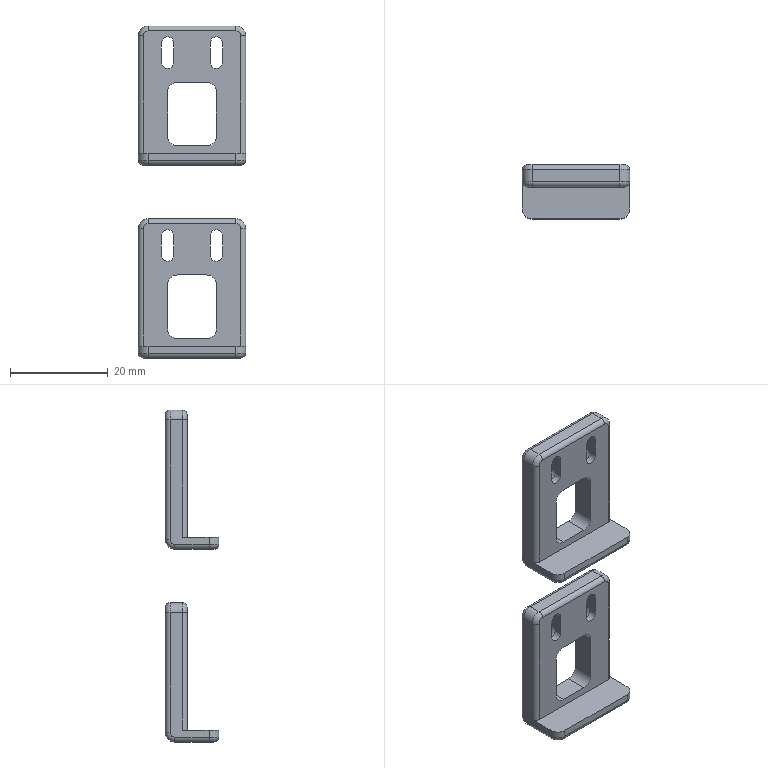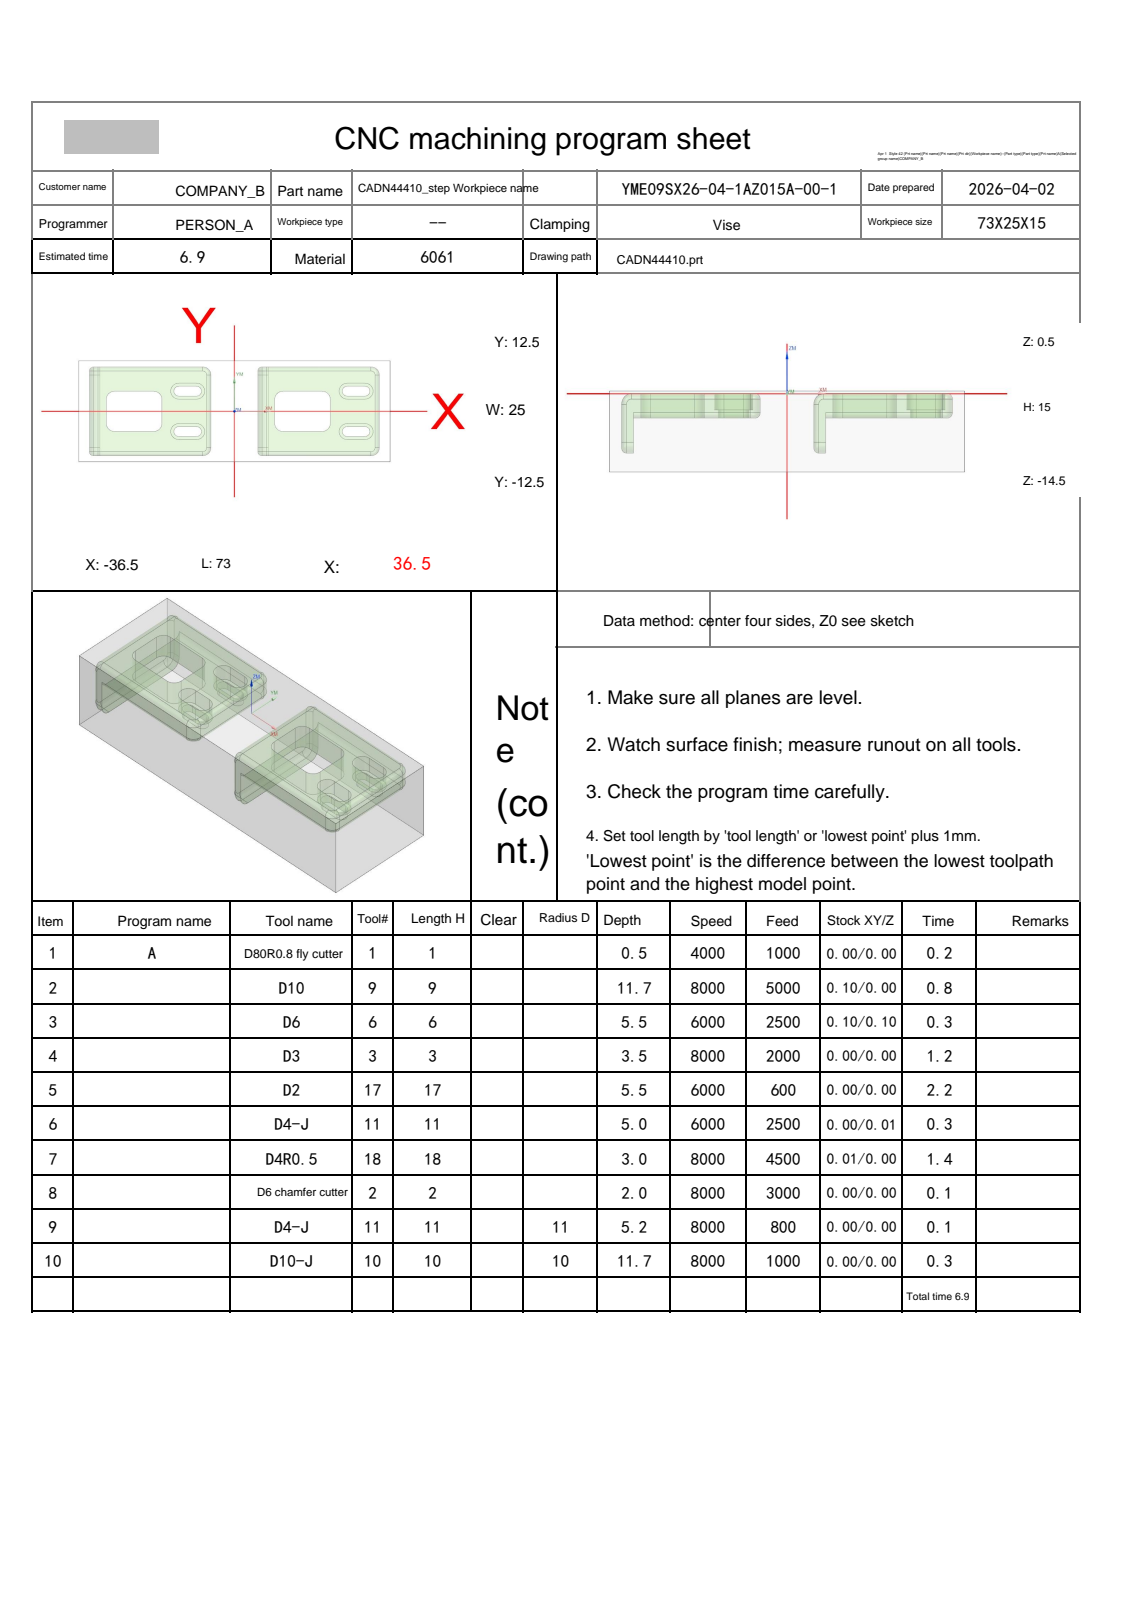NC program | NX | posted by the shop | part box 22 x 11 x 68 mm
Lines 3075 to 4128 of 7842:
N6 T11 M06
(D4-J  D=4. R=0. H=11 ce=0.00 di=0.01)
G00 G90 G54 X-26.358 Y2.4 M03 S6000
G43 H11 Z20.
M08
Z.319
G01 X-26.359 Y2.407 Z.233 F2000.
X-26.362 Y2.426 Z.155
X-26.367 Y2.455 Z.085
X-26.375 Y2.494 Z.023
X-26.386 Y2.539 Z-.033
X-26.4 Y2.59 Z-.082
X-26.417 Y2.644 Z-.125
X-26.438 Y2.7 Z-.161
X-26.462 Y2.756 Z-.192
X-26.49 Y2.81 Z-.218
X-26.523 Y2.861 Z-.239
X-26.56 Y2.906 Z-.255
X-26.602 Y2.945 Z-.267
X-26.648 Y2.974 Z-.275
X-26.7 Y2.993 Z-.28
X-26.758 Y3. Z-.281
X-28.05 F2500.
Y1.708
X-28.035 Y1.649 Z-.283
X-27.992 Y1.607 Z-.286
X-27.925 Y1.58 Z-.292
X-27.841 Y1.567 Z-.3
X-27.742 Y1.565 Z-.309
X-27.635 Y1.574 Z-.319
X-27.523 Y1.593 Z-.331
X-27.411 Y1.62 Z-.344
X-27.304 Y1.653 Z-.357
X-27.133 Y1.728 Z-.383
X-26.99 Y1.823 Z-.409
X-26.873 Y1.941 Z-.435
X-26.778 Y2.083 Z-.461
X-26.703 Y2.254 Z-.486
X-26.669 Y2.361 Z-.5
X-26.642 Y2.473 Z-.512
X-26.624 Y2.585 Z-.524
X-26.614 Y2.692 Z-.535
X-26.616 Y2.791 Z-.544
X-26.63 Y2.875 Z-.552
X-26.657 Y2.942 Z-.558
X-26.699 Y2.985 Z-.561
X-26.757 Y3. Z-.562
X-28.05
Y1.707
X-28.035 Y1.649 Z-.564
X-27.991 Y1.607 Z-.567
X-27.925 Y1.58 Z-.573
X-27.84 Y1.566 Z-.581
X-27.742 Y1.564 Z-.59
X-27.634 Y1.574 Z-.601
X-27.522 Y1.592 Z-.613
X-27.41 Y1.619 Z-.625
X-27.302 Y1.653 Z-.639
X-27.131 Y1.728 Z-.664
X-26.988 Y1.823 Z-.69
X-26.869 Y1.94 Z-.716
X-26.774 Y2.083 Z-.742
X-26.699 Y2.254 Z-.768
X-26.665 Y2.361 Z-.781
X-26.638 Y2.473 Z-.794
X-26.619 Y2.585 Z-.806
X-26.609 Y2.692 Z-.816
X-26.611 Y2.791 Z-.825
X-26.624 Y2.875 Z-.833
X-26.651 Y2.941 Z-.839
X-26.693 Y2.985 Z-.842
X-26.751 Y3. Z-.844
X-28.05
Y1.701
X-28.035 Y1.643 Z-.845
X-27.991 Y1.601 Z-.849
X-27.925 Y1.574 Z-.854
X-27.84 Y1.561 Z-.862
X-27.742 Y1.559 Z-.871
X-27.634 Y1.569 Z-.882
X-27.522 Y1.588 Z-.894
X-27.41 Y1.615 Z-.907
X-27.302 Y1.649 Z-.92
X-27.131 Y1.724 Z-.945
X-26.988 Y1.819 Z-.971
X-26.869 Y1.938 Z-.998
X-26.774 Y2.081 Z-1.024
X-26.699 Y2.252 Z-1.049
X-26.665 Y2.36 Z-1.062
X-26.638 Y2.472 Z-1.075
X-26.619 Y2.584 Z-1.087
X-26.609 Y2.692 Z-1.097
X-26.611 Y2.79 Z-1.107
X-26.624 Y2.875 Z-1.114
X-26.651 Y2.941 Z-1.12
X-26.693 Y2.985 Z-1.124
X-26.751 Y3. Z-1.125
X-28.05
Y1.701
X-28.035 Y1.643 Z-1.126
X-27.991 Y1.601 Z-1.13
X-27.925 Y1.574 Z-1.136
X-27.84 Y1.561 Z-1.143
X-27.742 Y1.559 Z-1.153
X-27.634 Y1.569 Z-1.163
X-27.522 Y1.588 Z-1.175
X-27.41 Y1.615 Z-1.188
X-27.302 Y1.649 Z-1.201
X-27.131 Y1.724 Z-1.226
X-26.988 Y1.819 Z-1.252
X-26.869 Y1.938 Z-1.279
X-26.774 Y2.081 Z-1.305
X-26.699 Y2.252 Z-1.33
X-26.665 Y2.36 Z-1.343
X-26.638 Y2.472 Z-1.356
X-26.619 Y2.584 Z-1.368
X-26.609 Y2.692 Z-1.379
X-26.611 Y2.79 Z-1.388
X-26.624 Y2.875 Z-1.396
X-26.651 Y2.941 Z-1.401
X-26.693 Y2.985 Z-1.405
X-26.751 Y3. Z-1.406
X-28.05
Y1.701
X-28.035 Y1.643 Z-1.408
X-27.991 Y1.601 Z-1.411
X-27.925 Y1.574 Z-1.417
X-27.84 Y1.561 Z-1.425
X-27.742 Y1.559 Z-1.434
X-27.634 Y1.569 Z-1.444
X-27.522 Y1.588 Z-1.456
X-27.41 Y1.615 Z-1.469
X-27.302 Y1.649 Z-1.482
X-27.131 Y1.724 Z-1.508
X-26.988 Y1.819 Z-1.534
X-26.869 Y1.938 Z-1.56
X-26.774 Y2.081 Z-1.586
X-26.699 Y2.252 Z-1.611
X-26.665 Y2.36 Z-1.625
X-26.638 Y2.472 Z-1.637
X-26.619 Y2.584 Z-1.649
X-26.609 Y2.692 Z-1.66
X-26.611 Y2.79 Z-1.669
X-26.624 Y2.875 Z-1.677
X-26.651 Y2.941 Z-1.683
X-26.693 Y2.985 Z-1.686
X-26.751 Y3. Z-1.688
X-28.05
Y1.701
X-28.035 Y1.643 Z-1.689
X-27.991 Y1.601 Z-1.692
X-27.925 Y1.574 Z-1.698
X-27.84 Y1.561 Z-1.706
X-27.742 Y1.559 Z-1.715
X-27.634 Y1.569 Z-1.726
X-27.522 Y1.588 Z-1.738
X-27.41 Y1.615 Z-1.75
X-27.302 Y1.649 Z-1.764
X-27.131 Y1.724 Z-1.789
X-26.988 Y1.819 Z-1.815
X-26.869 Y1.938 Z-1.841
X-26.774 Y2.081 Z-1.867
X-26.699 Y2.252 Z-1.893
X-26.665 Y2.36 Z-1.906
X-26.638 Y2.472 Z-1.919
X-26.619 Y2.584 Z-1.931
X-26.609 Y2.692 Z-1.941
X-26.611 Y2.79 Z-1.95
X-26.624 Y2.875 Z-1.958
X-26.651 Y2.941 Z-1.964
X-26.693 Y2.985 Z-1.967
X-26.751 Y3. Z-1.969
X-28.05
Y1.701
X-28.035 Y1.643 Z-1.97
X-27.991 Y1.601 Z-1.974
X-27.925 Y1.574 Z-1.979
X-27.84 Y1.561 Z-1.987
X-27.742 Y1.559 Z-1.996
X-27.634 Y1.569 Z-2.007
X-27.522 Y1.588 Z-2.019
X-27.41 Y1.615 Z-2.032
X-27.302 Y1.649 Z-2.045
X-27.131 Y1.724 Z-2.07
X-26.988 Y1.819 Z-2.096
X-26.869 Y1.938 Z-2.123
X-26.774 Y2.081 Z-2.149
X-26.699 Y2.252 Z-2.174
X-26.665 Y2.36 Z-2.187
X-26.638 Y2.472 Z-2.2
X-26.619 Y2.584 Z-2.212
X-26.609 Y2.692 Z-2.222
X-26.611 Y2.79 Z-2.232
X-26.624 Y2.875 Z-2.239
X-26.651 Y2.941 Z-2.245
X-26.693 Y2.985 Z-2.249
X-26.751 Y3. Z-2.25
X-28.049
X-28.05 Y1.701
X-28.035 Y1.643 Z-2.251
X-27.991 Y1.601 Z-2.255
X-27.925 Y1.574 Z-2.261
X-27.84 Y1.561 Z-2.268
X-27.742 Y1.559 Z-2.278
X-27.634 Y1.569 Z-2.288
X-27.522 Y1.588 Z-2.3
X-27.41 Y1.615 Z-2.313
X-27.302 Y1.649 Z-2.326
X-27.131 Y1.724 Z-2.351
X-26.988 Y1.819 Z-2.377
X-26.869 Y1.938 Z-2.404
X-26.774 Y2.081 Z-2.43
X-26.699 Y2.252 Z-2.455
X-26.665 Y2.36 Z-2.468
X-26.638 Y2.472 Z-2.481
X-26.619 Y2.584 Z-2.493
X-26.609 Y2.692 Z-2.504
X-26.611 Y2.79 Z-2.513
X-26.624 Y2.875 Z-2.521
X-26.651 Y2.941 Z-2.526
X-26.693 Y2.985 Z-2.53
X-26.751 Y3. Z-2.531
X-28.049
X-28.05 Y1.701
X-28.035 Y1.643 Z-2.533
X-27.991 Y1.601 Z-2.536
X-27.925 Y1.574 Z-2.542
X-27.84 Y1.561 Z-2.55
X-27.742 Y1.559 Z-2.559
X-27.634 Y1.569 Z-2.569
X-27.522 Y1.588 Z-2.581
X-27.41 Y1.615 Z-2.594
X-27.302 Y1.649 Z-2.607
X-27.131 Y1.724 Z-2.633
X-26.988 Y1.819 Z-2.659
X-26.869 Y1.938 Z-2.685
X-26.774 Y2.081 Z-2.711
X-26.699 Y2.252 Z-2.736
X-26.665 Y2.36 Z-2.75
X-26.638 Y2.472 Z-2.762
X-26.619 Y2.584 Z-2.774
X-26.609 Y2.692 Z-2.785
X-26.611 Y2.79 Z-2.794
X-26.624 Y2.875 Z-2.802
X-26.651 Y2.941 Z-2.808
X-26.693 Y2.985 Z-2.811
X-26.751 Y3. Z-2.813
X-28.049
X-28.05 Y1.701
X-28.035 Y1.643 Z-2.814
X-27.991 Y1.601 Z-2.817
X-27.925 Y1.574 Z-2.823
X-27.84 Y1.561 Z-2.831
X-27.742 Y1.559 Z-2.84
X-27.634 Y1.569 Z-2.851
X-27.522 Y1.588 Z-2.863
X-27.41 Y1.615 Z-2.875
X-27.302 Y1.649 Z-2.889
X-27.131 Y1.724 Z-2.914
X-26.988 Y1.819 Z-2.94
X-26.869 Y1.938 Z-2.966
X-26.774 Y2.081 Z-2.992
X-26.699 Y2.252 Z-3.018
X-26.665 Y2.36 Z-3.031
X-26.638 Y2.472 Z-3.044
X-26.619 Y2.584 Z-3.056
X-26.609 Y2.692 Z-3.066
X-26.611 Y2.79 Z-3.075
X-26.624 Y2.875 Z-3.083
X-26.651 Y2.941 Z-3.089
X-26.693 Y2.985 Z-3.092
X-26.751 Y3. Z-3.094
X-28.049
X-28.05 Y1.701
X-28.035 Y1.643 Z-3.095
X-27.991 Y1.601 Z-3.099
X-27.925 Y1.574 Z-3.104
X-27.84 Y1.561 Z-3.112
X-27.742 Y1.559 Z-3.121
X-27.634 Y1.569 Z-3.132
X-27.522 Y1.588 Z-3.144
X-27.41 Y1.615 Z-3.157
X-27.302 Y1.649 Z-3.17
X-27.131 Y1.724 Z-3.195
X-26.988 Y1.819 Z-3.221
X-26.869 Y1.938 Z-3.248
X-26.774 Y2.081 Z-3.274
X-26.699 Y2.252 Z-3.299
X-26.665 Y2.36 Z-3.312
X-26.638 Y2.472 Z-3.325
X-26.619 Y2.584 Z-3.337
X-26.609 Y2.692 Z-3.347
X-26.611 Y2.79 Z-3.357
X-26.624 Y2.875 Z-3.364
X-26.651 Y2.941 Z-3.37
X-26.693 Y2.985 Z-3.374
X-26.751 Y3. Z-3.375
X-28.049
X-28.05 Y1.701
X-28.035 Y1.643 Z-3.376
X-27.991 Y1.601 Z-3.38
X-27.925 Y1.574 Z-3.386
X-27.84 Y1.561 Z-3.393
X-27.742 Y1.559 Z-3.403
X-27.634 Y1.569 Z-3.413
X-27.522 Y1.588 Z-3.425
X-27.41 Y1.615 Z-3.438
X-27.302 Y1.649 Z-3.451
X-27.131 Y1.724 Z-3.476
X-26.988 Y1.819 Z-3.502
X-26.869 Y1.938 Z-3.529
X-26.774 Y2.081 Z-3.555
X-26.699 Y2.252 Z-3.58
X-26.665 Y2.36 Z-3.593
X-26.638 Y2.472 Z-3.606
X-26.619 Y2.584 Z-3.618
X-26.609 Y2.692 Z-3.629
X-26.611 Y2.79 Z-3.638
X-26.624 Y2.875 Z-3.646
X-26.651 Y2.941 Z-3.651
X-26.693 Y2.985 Z-3.655
X-26.751 Y3. Z-3.656
X-28.049
X-28.05 Y1.701
X-28.035 Y1.643 Z-3.658
X-27.991 Y1.601 Z-3.661
X-27.925 Y1.574 Z-3.667
X-27.84 Y1.561 Z-3.675
X-27.742 Y1.559 Z-3.684
X-27.634 Y1.569 Z-3.694
X-27.522 Y1.588 Z-3.706
X-27.41 Y1.615 Z-3.719
X-27.302 Y1.649 Z-3.732
X-27.131 Y1.724 Z-3.758
X-26.988 Y1.819 Z-3.784
X-26.869 Y1.938 Z-3.81
X-26.774 Y2.081 Z-3.836
X-26.699 Y2.252 Z-3.861
X-26.665 Y2.36 Z-3.875
X-26.638 Y2.472 Z-3.887
X-26.619 Y2.584 Z-3.899
X-26.609 Y2.692 Z-3.91
X-26.611 Y2.79 Z-3.919
X-26.624 Y2.875 Z-3.927
X-26.651 Y2.941 Z-3.933
X-26.693 Y2.985 Z-3.936
X-26.751 Y3. Z-3.938
X-28.049
X-28.05 Y1.701
X-28.035 Y1.643 Z-3.939
X-27.991 Y1.601 Z-3.942
X-27.925 Y1.574 Z-3.948
X-27.84 Y1.561 Z-3.956
X-27.742 Y1.559 Z-3.965
X-27.634 Y1.569 Z-3.976
X-27.522 Y1.588 Z-3.988
X-27.41 Y1.615 Z-4.
X-27.302 Y1.649 Z-4.014
X-27.131 Y1.724 Z-4.039
X-26.988 Y1.819 Z-4.065
X-26.869 Y1.938 Z-4.091
X-26.774 Y2.081 Z-4.117
X-26.699 Y2.252 Z-4.143
X-26.665 Y2.36 Z-4.156
X-26.638 Y2.472 Z-4.169
X-26.619 Y2.584 Z-4.181
X-26.609 Y2.692 Z-4.191
X-26.611 Y2.79 Z-4.2
X-26.624 Y2.875 Z-4.208
X-26.651 Y2.941 Z-4.214
X-26.693 Y2.985 Z-4.217
X-26.751 Y3. Z-4.219
X-28.049
X-28.05 Y1.701
X-28.035 Y1.643 Z-4.22
X-27.991 Y1.601 Z-4.224
X-27.925 Y1.574 Z-4.229
X-27.84 Y1.561 Z-4.237
X-27.742 Y1.559 Z-4.246
X-27.634 Y1.569 Z-4.257
X-27.522 Y1.588 Z-4.269
X-27.41 Y1.615 Z-4.282
X-27.302 Y1.649 Z-4.295
X-27.131 Y1.724 Z-4.32
X-26.988 Y1.819 Z-4.346
X-26.869 Y1.938 Z-4.373
X-26.774 Y2.081 Z-4.399
X-26.699 Y2.252 Z-4.424
X-26.665 Y2.36 Z-4.437
X-26.638 Y2.472 Z-4.45
X-26.619 Y2.584 Z-4.462
X-26.609 Y2.692 Z-4.472
X-26.611 Y2.79 Z-4.482
X-26.624 Y2.875 Z-4.489
X-26.651 Y2.941 Z-4.495
X-26.693 Y2.985 Z-4.499
X-26.751 Y3. Z-4.5
X-28.049
X-28.05 Y1.701
X-28.041 Y1.634 Z-4.485
X-28.018 Y1.556 Z-4.44
X-27.981 Y1.466 Z-4.369
X-27.935 Y1.367 Z-4.275
X-27.881 Y1.259 Z-4.159
X-27.791 Y1.08 Z-3.945
X-27.732 Y.959 Z-3.79
X-27.649 Y.773 Z-3.539
X-27.6 Y.644 Z-3.357
X-27.528 Y.386 Z-2.979
X-27.492 Y.126 Z-2.588
Y-.133 Z-2.193
X-27.528 Y-.393 Z-1.802
X-27.6 Y-.652 Z-1.424
X-27.649 Y-.78 Z-1.242
X-27.732 Y-.967 Z-.991
X-27.791 Y-1.088 Z-.836
X-27.881 Y-1.266 Z-.622
X-27.935 Y-1.374 Z-.506
X-27.981 Y-1.473 Z-.412
X-28.018 Y-1.563 Z-.341
X-28.041 Y-1.642 Z-.297
X-28.05 Y-1.708 Z-.281
Y-3.
X-26.758
X-26.7 Y-2.985 Z-.283
X-26.658 Y-2.942 Z-.286
X-26.631 Y-2.875 Z-.292
X-26.617 Y-2.791 Z-.3
X-26.616 Y-2.693 Z-.309
X-26.625 Y-2.585 Z-.319
X-26.644 Y-2.473 Z-.331
X-26.67 Y-2.361 Z-.344
X-26.704 Y-2.254 Z-.357
X-26.779 Y-2.084 Z-.383
X-26.873 Y-1.941 Z-.409
X-26.991 Y-1.823 Z-.435
X-27.134 Y-1.728 Z-.461
X-27.304 Y-1.654 Z-.486
X-27.411 Y-1.62 Z-.5
X-27.523 Y-1.594 Z-.512
X-27.635 Y-1.575 Z-.524
X-27.743 Y-1.566 Z-.535
X-27.841 Y-1.567 Z-.544
X-27.925 Y-1.581 Z-.552
X-27.992 Y-1.608 Z-.558
X-28.035 Y-1.65 Z-.561
X-28.05 Y-1.708 Z-.562
Y-3.
X-26.758
X-26.7 Y-2.985 Z-.564
X-26.658 Y-2.942 Z-.567
X-26.631 Y-2.875 Z-.573
X-26.617 Y-2.791 Z-.581
X-26.616 Y-2.692 Z-.59
X-26.625 Y-2.585 Z-.601
X-26.644 Y-2.473 Z-.613
X-26.67 Y-2.361 Z-.625
X-26.704 Y-2.254 Z-.639
X-26.778 Y-2.083 Z-.664
X-26.873 Y-1.941 Z-.69
X-26.991 Y-1.823 Z-.716
X-27.134 Y-1.728 Z-.742
X-27.304 Y-1.654 Z-.768
X-27.411 Y-1.62 Z-.781
X-27.523 Y-1.593 Z-.794
X-27.635 Y-1.575 Z-.806
X-27.743 Y-1.565 Z-.816
X-27.841 Y-1.567 Z-.825
X-27.925 Y-1.581 Z-.833
X-27.992 Y-1.608 Z-.839
X-28.035 Y-1.65 Z-.842
X-28.05 Y-1.708 Z-.844
Y-3.
X-26.758
X-26.7 Y-2.985 Z-.845
X-26.658 Y-2.942 Z-.849
X-26.631 Y-2.875 Z-.854
X-26.617 Y-2.791 Z-.862
X-26.615 Y-2.692 Z-.871
X-26.625 Y-2.585 Z-.882
X-26.643 Y-2.473 Z-.894
X-26.67 Y-2.361 Z-.907
X-26.704 Y-2.254 Z-.92
X-26.778 Y-2.083 Z-.945
X-26.873 Y-1.941 Z-.971
X-26.991 Y-1.823 Z-.998
X-27.133 Y-1.728 Z-1.024
X-27.304 Y-1.654 Z-1.049
X-27.411 Y-1.62 Z-1.062
X-27.523 Y-1.593 Z-1.075
X-27.635 Y-1.575 Z-1.087
X-27.743 Y-1.565 Z-1.097
X-27.841 Y-1.567 Z-1.107
X-27.925 Y-1.58 Z-1.114
X-27.992 Y-1.608 Z-1.12
X-28.035 Y-1.65 Z-1.124
X-28.05 Y-1.708 Z-1.125
Y-3.
X-26.758
X-26.7 Y-2.985 Z-1.126
X-26.658 Y-2.942 Z-1.13
X-26.631 Y-2.875 Z-1.136
X-26.617 Y-2.791 Z-1.143
X-26.615 Y-2.692 Z-1.153
X-26.625 Y-2.585 Z-1.163
X-26.643 Y-2.473 Z-1.175
X-26.67 Y-2.361 Z-1.188
X-26.704 Y-2.254 Z-1.201
X-26.778 Y-2.083 Z-1.226
X-26.873 Y-1.941 Z-1.252
X-26.991 Y-1.823 Z-1.279
X-27.133 Y-1.728 Z-1.305
X-27.304 Y-1.653 Z-1.33
X-27.411 Y-1.62 Z-1.343
X-27.523 Y-1.593 Z-1.356
X-27.635 Y-1.574 Z-1.368
X-27.742 Y-1.565 Z-1.379
X-27.841 Y-1.567 Z-1.388
X-27.925 Y-1.58 Z-1.396
X-27.992 Y-1.607 Z-1.401
X-28.035 Y-1.649 Z-1.405
X-28.05 Y-1.708 Z-1.406
Y-3.
X-26.758
X-26.699 Y-2.985 Z-1.408
X-26.657 Y-2.942 Z-1.411
X-26.63 Y-2.875 Z-1.417
X-26.617 Y-2.791 Z-1.425
X-26.615 Y-2.692 Z-1.434
X-26.624 Y-2.585 Z-1.444
X-26.643 Y-2.473 Z-1.456
X-26.67 Y-2.361 Z-1.469
X-26.703 Y-2.254 Z-1.482
X-26.778 Y-2.083 Z-1.508
X-26.873 Y-1.94 Z-1.534
X-26.991 Y-1.823 Z-1.56
X-27.133 Y-1.728 Z-1.586
X-27.304 Y-1.653 Z-1.611
X-27.411 Y-1.62 Z-1.625
X-27.523 Y-1.593 Z-1.637
X-27.635 Y-1.574 Z-1.649
X-27.742 Y-1.565 Z-1.66
X-27.841 Y-1.567 Z-1.669
X-27.925 Y-1.58 Z-1.677
X-27.992 Y-1.607 Z-1.683
X-28.035 Y-1.649 Z-1.686
X-28.05 Y-1.707 Z-1.688
Y-3.
X-26.757
X-26.699 Y-2.985 Z-1.689
X-26.657 Y-2.942 Z-1.692
X-26.63 Y-2.875 Z-1.698
X-26.617 Y-2.791 Z-1.706
X-26.615 Y-2.692 Z-1.715
X-26.624 Y-2.585 Z-1.726
X-26.643 Y-2.473 Z-1.738
X-26.67 Y-2.361 Z-1.75
X-26.703 Y-2.254 Z-1.764
X-26.778 Y-2.083 Z-1.789
X-26.873 Y-1.94 Z-1.815
X-26.99 Y-1.823 Z-1.841
X-27.133 Y-1.728 Z-1.867
X-27.304 Y-1.653 Z-1.893
X-27.411 Y-1.62 Z-1.906
X-27.523 Y-1.593 Z-1.919
X-27.635 Y-1.574 Z-1.931
X-27.742 Y-1.565 Z-1.941
X-27.841 Y-1.566 Z-1.95
X-27.925 Y-1.58 Z-1.958
X-27.992 Y-1.607 Z-1.964
X-28.035 Y-1.649 Z-1.967
X-28.05 Y-1.707 Z-1.969
Y-2.999
X-26.757 Y-3.
X-26.699 Y-2.985 Z-1.97
X-26.657 Y-2.942 Z-1.974
X-26.63 Y-2.875 Z-1.979
X-26.616 Y-2.791 Z-1.987
X-26.615 Y-2.692 Z-1.996
X-26.624 Y-2.585 Z-2.007
X-26.643 Y-2.473 Z-2.019
X-26.67 Y-2.361 Z-2.032
X-26.703 Y-2.254 Z-2.045
X-26.778 Y-2.083 Z-2.07
X-26.873 Y-1.94 Z-2.096
X-26.99 Y-1.823 Z-2.123
X-27.133 Y-1.728 Z-2.149
X-27.304 Y-1.653 Z-2.174
X-27.411 Y-1.62 Z-2.187
X-27.523 Y-1.593 Z-2.2
X-27.635 Y-1.574 Z-2.212
X-27.742 Y-1.565 Z-2.222
X-27.841 Y-1.566 Z-2.232
X-27.925 Y-1.58 Z-2.239
X-27.992 Y-1.607 Z-2.245
X-28.035 Y-1.649 Z-2.249
X-28.05 Y-1.707 Z-2.25
Y-2.999
X-26.757 Y-3.
X-26.699 Y-2.985 Z-2.251
X-26.657 Y-2.942 Z-2.255
X-26.63 Y-2.875 Z-2.261
X-26.616 Y-2.791 Z-2.268
X-26.615 Y-2.692 Z-2.278
X-26.624 Y-2.585 Z-2.288
X-26.643 Y-2.473 Z-2.3
X-26.67 Y-2.361 Z-2.313
X-26.703 Y-2.254 Z-2.326
X-26.778 Y-2.083 Z-2.351
X-26.873 Y-1.94 Z-2.377
X-26.99 Y-1.823 Z-2.404
X-27.133 Y-1.728 Z-2.43
X-27.304 Y-1.653 Z-2.455
X-27.411 Y-1.619 Z-2.468
X-27.523 Y-1.593 Z-2.481
X-27.635 Y-1.574 Z-2.493
X-27.742 Y-1.565 Z-2.504
X-27.841 Y-1.566 Z-2.513
X-27.925 Y-1.58 Z-2.521
X-27.992 Y-1.607 Z-2.526
X-28.035 Y-1.649 Z-2.53
X-28.05 Y-1.707 Z-2.531
Y-2.999
X-26.757 Y-3.
X-26.699 Y-2.985 Z-2.533
X-26.657 Y-2.941 Z-2.536
X-26.63 Y-2.875 Z-2.542
X-26.616 Y-2.791 Z-2.55
X-26.615 Y-2.692 Z-2.559
X-26.624 Y-2.585 Z-2.569
X-26.643 Y-2.473 Z-2.581
X-26.669 Y-2.361 Z-2.594
X-26.703 Y-2.254 Z-2.607
X-26.778 Y-2.083 Z-2.633
X-26.873 Y-1.94 Z-2.659
X-26.99 Y-1.823 Z-2.685
X-27.133 Y-1.728 Z-2.711
X-27.304 Y-1.653 Z-2.736
X-27.411 Y-1.619 Z-2.75
X-27.523 Y-1.592 Z-2.762
X-27.635 Y-1.574 Z-2.774
X-27.742 Y-1.564 Z-2.785
X-27.841 Y-1.566 Z-2.794
X-27.925 Y-1.58 Z-2.802
X-27.992 Y-1.607 Z-2.808
X-28.035 Y-1.649 Z-2.811
X-28.05 Y-1.707 Z-2.813
Y-2.999
X-26.757 Y-3.
X-26.699 Y-2.985 Z-2.814
X-26.657 Y-2.941 Z-2.817
X-26.63 Y-2.875 Z-2.823
X-26.616 Y-2.791 Z-2.831
X-26.614 Y-2.692 Z-2.84
X-26.624 Y-2.585 Z-2.851
X-26.643 Y-2.473 Z-2.863
X-26.669 Y-2.361 Z-2.875
X-26.703 Y-2.254 Z-2.889
X-26.778 Y-2.083 Z-2.914
X-26.873 Y-1.94 Z-2.94
X-26.99 Y-1.823 Z-2.966
X-27.133 Y-1.728 Z-2.992
X-27.304 Y-1.653 Z-3.018
X-27.411 Y-1.619 Z-3.031
X-27.523 Y-1.592 Z-3.044
X-27.635 Y-1.574 Z-3.056
X-27.742 Y-1.564 Z-3.066
X-27.841 Y-1.566 Z-3.075
X-27.925 Y-1.579 Z-3.083
X-27.992 Y-1.607 Z-3.089
X-28.035 Y-1.648 Z-3.092
X-28.05 Y-1.707 Z-3.094
Y-2.999
X-26.757 Y-3.
X-26.699 Y-2.985 Z-3.095
X-26.657 Y-2.941 Z-3.099
X-26.629 Y-2.875 Z-3.104
X-26.616 Y-2.791 Z-3.112
X-26.614 Y-2.692 Z-3.121
X-26.624 Y-2.585 Z-3.132
X-26.642 Y-2.473 Z-3.144
X-26.669 Y-2.361 Z-3.157
X-26.703 Y-2.254 Z-3.17
X-26.778 Y-2.083 Z-3.195
X-26.873 Y-1.94 Z-3.221
X-26.99 Y-1.822 Z-3.248
X-27.133 Y-1.727 Z-3.274
X-27.304 Y-1.653 Z-3.299
X-27.411 Y-1.619 Z-3.312
X-27.523 Y-1.592 Z-3.325
X-27.635 Y-1.573 Z-3.337
X-27.742 Y-1.564 Z-3.347
X-27.841 Y-1.566 Z-3.357
X-27.925 Y-1.579 Z-3.364
X-27.992 Y-1.606 Z-3.37
X-28.035 Y-1.648 Z-3.374
X-28.05 Y-1.706 Z-3.375
Y-2.999
X-26.756 Y-3.
X-26.698 Y-2.985 Z-3.376
X-26.656 Y-2.941 Z-3.38
X-26.629 Y-2.875 Z-3.386
X-26.616 Y-2.791 Z-3.393
X-26.614 Y-2.692 Z-3.403
X-26.624 Y-2.585 Z-3.413
X-26.642 Y-2.473 Z-3.425
X-26.669 Y-2.361 Z-3.438
X-26.703 Y-2.254 Z-3.451
X-26.778 Y-2.083 Z-3.476
X-26.872 Y-1.94 Z-3.502
X-26.99 Y-1.822 Z-3.529
X-27.133 Y-1.727 Z-3.555
X-27.304 Y-1.653 Z-3.58
X-27.411 Y-1.619 Z-3.593
X-27.523 Y-1.592 Z-3.606
X-27.635 Y-1.573 Z-3.618
X-27.742 Y-1.564 Z-3.629
X-27.841 Y-1.566 Z-3.638
X-27.925 Y-1.579 Z-3.646
X-27.992 Y-1.606 Z-3.651
X-28.035 Y-1.648 Z-3.655
X-28.05 Y-1.706 Z-3.656
Y-2.999
X-26.756 Y-3.
X-26.698 Y-2.985 Z-3.658
X-26.656 Y-2.941 Z-3.661
X-26.629 Y-2.875 Z-3.667
X-26.616 Y-2.79 Z-3.675
X-26.614 Y-2.692 Z-3.684
X-26.623 Y-2.584 Z-3.694
X-26.642 Y-2.472 Z-3.706
X-26.669 Y-2.36 Z-3.719
X-26.703 Y-2.252 Z-3.732
X-26.777 Y-2.081 Z-3.758
X-26.872 Y-1.938 Z-3.784
X-26.99 Y-1.819 Z-3.81
X-27.133 Y-1.724 Z-3.836
X-27.304 Y-1.649 Z-3.861
X-27.411 Y-1.615 Z-3.875
X-27.523 Y-1.588 Z-3.887
X-27.635 Y-1.569 Z-3.899
X-27.742 Y-1.559 Z-3.91
X-27.841 Y-1.561 Z-3.919
X-27.925 Y-1.574 Z-3.927
X-27.992 Y-1.601 Z-3.933
X-28.035 Y-1.643 Z-3.936
X-28.05 Y-1.701 Z-3.938
X-28.049 Y-3.
X-26.751
X-26.693 Y-2.985 Z-3.939
X-26.651 Y-2.941 Z-3.942
X-26.624 Y-2.875 Z-3.948
X-26.611 Y-2.79 Z-3.956
X-26.609 Y-2.692 Z-3.965
X-26.619 Y-2.584 Z-3.976
X-26.638 Y-2.472 Z-3.988
X-26.665 Y-2.36 Z-4.
X-26.699 Y-2.252 Z-4.014
X-26.774 Y-2.081 Z-4.039
X-26.869 Y-1.938 Z-4.065
X-26.988 Y-1.819 Z-4.091
X-27.131 Y-1.724 Z-4.117
X-27.302 Y-1.649 Z-4.143
X-27.41 Y-1.615 Z-4.156
X-27.522 Y-1.588 Z-4.169
X-27.634 Y-1.569 Z-4.181
X-27.742 Y-1.559 Z-4.191
X-27.84 Y-1.561 Z-4.2
X-27.925 Y-1.574 Z-4.208
X-27.991 Y-1.601 Z-4.214
X-28.035 Y-1.643 Z-4.217
X-28.05 Y-1.701 Z-4.219
X-28.049 Y-3.
X-26.751
X-26.693 Y-2.985 Z-4.22
X-26.651 Y-2.941 Z-4.224
X-26.624 Y-2.875 Z-4.229
X-26.611 Y-2.79 Z-4.237
X-26.609 Y-2.692 Z-4.246
X-26.619 Y-2.584 Z-4.257
X-26.638 Y-2.472 Z-4.269
X-26.665 Y-2.36 Z-4.282
X-26.699 Y-2.252 Z-4.295
X-26.774 Y-2.081 Z-4.32
X-26.869 Y-1.938 Z-4.346
X-26.988 Y-1.819 Z-4.373
X-27.131 Y-1.724 Z-4.399
X-27.302 Y-1.649 Z-4.424
X-27.41 Y-1.615 Z-4.437
X-27.522 Y-1.588 Z-4.45
X-27.634 Y-1.569 Z-4.462
X-27.742 Y-1.559 Z-4.472
X-27.84 Y-1.561 Z-4.482
X-27.925 Y-1.574 Z-4.489
X-27.991 Y-1.601 Z-4.495
X-28.035 Y-1.643 Z-4.499
X-28.05 Y-1.701 Z-4.5
X-28.049 Y-3.
X-26.751
X-26.682 Y-2.993 Z-4.487
X-26.585 Y-2.973 Z-4.45
X-26.463 Y-2.942 Z-4.391
X-26.07 Y-2.833 Z-4.162
X-25.557 Y-2.699 Z-3.828
X-24.87 Y-2.55 Z-3.357
X-24.339 Y-2.478 Z-2.979
X-23.797 Y-2.442 Z-2.588
X-23.253 Z-2.193
X-22.711 Y-2.478 Z-1.802
X-22.18 Y-2.55 Z-1.424
X-21.493 Y-2.699 Z-.953
X-20.98 Y-2.833 Z-.62
X-20.587 Y-2.942 Z-.39
X-20.465 Y-2.973 Z-.331
X-20.368 Y-2.993 Z-.294
X-20.299 Y-3. Z-.281
X-19.
Y-1.701
X-19.015 Y-1.643 Z-.283
X-19.059 Y-1.601 Z-.286
X-19.125 Y-1.574 Z-.292
X-19.21 Y-1.561 Z-.3
X-19.309 Y-1.559 Z-.309
X-19.417 Y-1.569 Z-.319
X-19.529 Y-1.588 Z-.331
X-19.642 Y-1.615 Z-.344
X-19.749 Y-1.649 Z-.357
X-19.921 Y-1.724 Z-.383
X-20.064 Y-1.819 Z-.409
X-20.182 Y-1.938 Z-.435
X-20.277 Y-2.081 Z-.461
X-20.352 Y-2.252 Z-.486
X-20.386 Y-2.36 Z-.5
X-20.413 Y-2.472 Z-.512
X-20.432 Y-2.584 Z-.524
X-20.441 Y-2.692 Z-.535
X-20.44 Y-2.79 Z-.544
X-20.426 Y-2.875 Z-.552
X-20.399 Y-2.941 Z-.558
X-20.357 Y-2.985 Z-.561
X-20.299 Y-3. Z-.562
X-19.
Y-1.701
X-19.016 Y-1.643 Z-.564
X-19.059 Y-1.601 Z-.567
X-19.126 Y-1.574 Z-.573
X-19.212 Y-1.561 Z-.581
X-19.311 Y-1.559 Z-.59
X-19.42 Y-1.569 Z-.6
X-19.533 Y-1.588 Z-.612
X-19.646 Y-1.615 Z-.625
X-19.754 Y-1.649 Z-.638
X-19.926 Y-1.724 Z-.663
X-20.069 Y-1.82 Z-.689
X-20.186 Y-1.938 Z-.716
X-20.281 Y-2.081 Z-.742
X-20.355 Y-2.253 Z-.767
X-20.388 Y-2.36 Z-.781
X-20.415 Y-2.472 Z-.794
X-20.433 Y-2.584 Z-.805
X-20.442 Y-2.692 Z-.816
X-20.44 Y-2.79 Z-.825
X-20.426 Y-2.875 Z-.833
X-20.399 Y-2.941 Z-.839
X-20.357 Y-2.985 Z-.842
X-20.299 Y-3. Z-.844
X-19.
Y-1.701
X-19.016 Y-1.643 Z-.845
X-19.059 Y-1.601 Z-.849
X-19.126 Y-1.574 Z-.854
X-19.212 Y-1.561 Z-.862
X-19.312 Y-1.56 Z-.871
X-19.42 Y-1.569 Z-.882
X-19.534 Y-1.588 Z-.893
X-19.647 Y-1.615 Z-.906
X-19.754 Y-1.649 Z-.919
X-19.926 Y-1.725 Z-.945
X-20.069 Y-1.82 Z-.971
X-20.187 Y-1.938 Z-.997
X-20.281 Y-2.081 Z-1.023
X-20.355 Y-2.253 Z-1.048
X-20.388 Y-2.36 Z-1.062
X-20.415 Y-2.472 Z-1.075
X-20.433 Y-2.584 Z-1.087
X-20.442 Y-2.692 Z-1.097
X-20.44 Y-2.79 Z-1.107
X-20.427 Y-2.875 Z-1.114
X-20.399 Y-2.941 Z-1.12
X-20.357 Y-2.985 Z-1.124
X-20.299 Y-3. Z-1.125
X-19.
Y-1.701
X-19.016 Y-1.643 Z-1.126
X-19.059 Y-1.601 Z-1.13
X-19.126 Y-1.574 Z-1.136
X-19.212 Y-1.561 Z-1.143
X-19.312 Y-1.56 Z-1.152
X-19.421 Y-1.569 Z-1.163
X-19.534 Y-1.588 Z-1.175
X-19.647 Y-1.615 Z-1.187
X-19.755 Y-1.649 Z-1.201
X-19.927 Y-1.725 Z-1.226
X-20.07 Y-1.82 Z-1.252
X-20.188 Y-1.938 Z-1.278
X-20.282 Y-2.082 Z-1.304
X-20.356 Y-2.253 Z-1.33
X-20.389 Y-2.36 Z-1.343
X-20.415 Y-2.472 Z-1.356
X-20.433 Y-2.584 Z-1.368
X-20.442 Y-2.692 Z-1.379
X-20.44 Y-2.79 Z-1.388
X-20.427 Y-2.875 Z-1.396
X-20.399 Y-2.941 Z-1.401
X-20.357 Y-2.985 Z-1.405
X-20.299 Y-3. Z-1.406
X-19.
Y-1.701
X-19.016 Y-1.643 Z-1.407
X-19.059 Y-1.601 Z-1.411
X-19.127 Y-1.574 Z-1.417
X-19.213 Y-1.561 Z-1.424
X-19.312 Y-1.56 Z-1.433
X-19.421 Y-1.569 Z-1.444
X-19.535 Y-1.589 Z-1.456
X-19.648 Y-1.616 Z-1.468
X-19.756 Y-1.65 Z-1.482
X-19.928 Y-1.725 Z-1.507
X-20.071 Y-1.821 Z-1.533
X-20.188 Y-1.939 Z-1.559
X-20.282 Y-2.082 Z-1.586
X-20.356 Y-2.253 Z-1.611
X-20.389 Y-2.36 Z-1.624
X-20.415 Y-2.472 Z-1.637
X-20.434 Y-2.584 Z-1.649
X-20.442 Y-2.692 Z-1.66
X-20.441 Y-2.791 Z-1.669
X-20.427 Y-2.875 Z-1.677
X-20.399 Y-2.941 Z-1.683
X-20.357 Y-2.985 Z-1.686
X-20.299 Y-3. Z-1.688
X-19.
Y-1.701
X-19.016 Y-1.643 Z-1.689
X-19.06 Y-1.601 Z-1.692
X-19.127 Y-1.574 Z-1.698
X-19.213 Y-1.561 Z-1.706
X-19.313 Y-1.56 Z-1.715
X-19.422 Y-1.57 Z-1.725
X-19.536 Y-1.589 Z-1.737
X-19.649 Y-1.616 Z-1.75
X-19.757 Y-1.65 Z-1.763
X-19.929 Y-1.726 Z-1.788
X-20.072 Y-1.821 Z-1.814
X-20.189 Y-1.939 Z-1.841
X-20.283 Y-2.082 Z-1.867
X-20.357 Y-2.253 Z-1.892
X-20.39 Y-2.36 Z-1.906
X-20.416 Y-2.472 Z-1.918
X-20.434 Y-2.584 Z-1.93
X-20.443 Y-2.692 Z-1.941
X-20.441 Y-2.791 Z-1.95
X-20.427 Y-2.875 Z-1.958
X-20.399 Y-2.941 Z-1.964
X-20.357 Y-2.985 Z-1.967
X-20.299 Y-3. Z-1.969
X-19.
Y-1.701
X-19.016 Y-1.643 Z-1.97
X-19.06 Y-1.601 Z-1.974
X-19.127 Y-1.574 Z-1.979
X-19.213 Y-1.561 Z-1.987
X-19.314 Y-1.56 Z-1.996
X-19.423 Y-1.57 Z-2.007
X-19.537 Y-1.589 Z-2.018
X-19.65 Y-1.617 Z-2.031
X-19.758 Y-1.651 Z-2.044
X-19.931 Y-1.726 Z-2.069
X-20.074 Y-1.821 Z-2.096
X-20.19 Y-1.939 Z-2.122
X-20.284 Y-2.082 Z-2.148
X-20.357 Y-2.253 Z-2.173
X-20.39 Y-2.361 Z-2.187
X-20.416 Y-2.473 Z-2.2
X-20.434 Y-2.585 Z-2.212
X-20.443 Y-2.692 Z-2.222
X-20.441 Y-2.791 Z-2.232
X-20.427 Y-2.875 Z-2.239
X-20.399 Y-2.941 Z-2.245
X-20.357 Y-2.985 Z-2.249
X-20.299 Y-3. Z-2.25
X-19.
Y-1.701
X-19.016 Y-1.643 Z-2.251
X-19.06 Y-1.601 Z-2.255
X-19.127 Y-1.575 Z-2.26
X-19.214 Y-1.561 Z-2.268
X-19.314 Y-1.56 Z-2.277
X-19.424 Y-1.57 Z-2.288
X-19.538 Y-1.59 Z-2.299
X-19.651 Y-1.617 Z-2.312
X-19.76 Y-1.651 Z-2.326
X-19.932 Y-1.727 Z-2.351
X-20.075 Y-1.822 Z-2.377
X-20.192 Y-1.94 Z-2.403
X-20.285 Y-2.083 Z-2.429
X-20.358 Y-2.254 Z-2.455
X-20.391 Y-2.361 Z-2.468
X-20.417 Y-2.473 Z-2.481
X-20.435 Y-2.585 Z-2.493
X-20.443 Y-2.692 Z-2.504
X-20.441 Y-2.791 Z-2.513
X-20.427 Y-2.875 Z-2.521
X-20.399 Y-2.941 Z-2.526
X-20.357 Y-2.985 Z-2.53
X-20.299 Y-3. Z-2.531
X-19.
Y-1.701
X-19.016 Y-1.643 Z-2.532
X-19.06 Y-1.601 Z-2.536
X-19.128 Y-1.575 Z-2.542
X-19.214 Y-1.562 Z-2.549
X-19.315 Y-1.561 Z-2.558
X-19.424 Y-1.571 Z-2.569
X-19.539 Y-1.59 Z-2.581
X-19.652 Y-1.618 Z-2.593
X-19.761 Y-1.652 Z-2.607
X-19.933 Y-1.727 Z-2.632
X-20.076 Y-1.823 Z-2.658
X-20.193 Y-1.94 Z-2.684
X-20.286 Y-2.083 Z-2.711
X-20.359 Y-2.254 Z-2.736
X-20.391 Y-2.361 Z-2.749
X-20.417 Y-2.473 Z-2.762
X-20.435 Y-2.585 Z-2.774
X-20.443 Y-2.692 Z-2.785
X-20.441 Y-2.791 Z-2.794
X-20.427 Y-2.875 Z-2.802
X-20.399 Y-2.942 Z-2.808
X-20.357 Y-2.985 Z-2.811
X-20.299 Y-3. Z-2.813
X-19.
Y-1.701
X-19.016 Y-1.643 Z-2.814
X-19.06 Y-1.601 Z-2.817
X-19.128 Y-1.575 Z-2.823
X-19.215 Y-1.562 Z-2.831
X-19.315 Y-1.561 Z-2.84
X-19.425 Y-1.571 Z-2.85
X-19.54 Y-1.591 Z-2.862
X-19.653 Y-1.618 Z-2.875
X-19.762 Y-1.652 Z-2.888
X-19.935 Y-1.728 Z-2.913
X-20.077 Y-1.823 Z-2.939